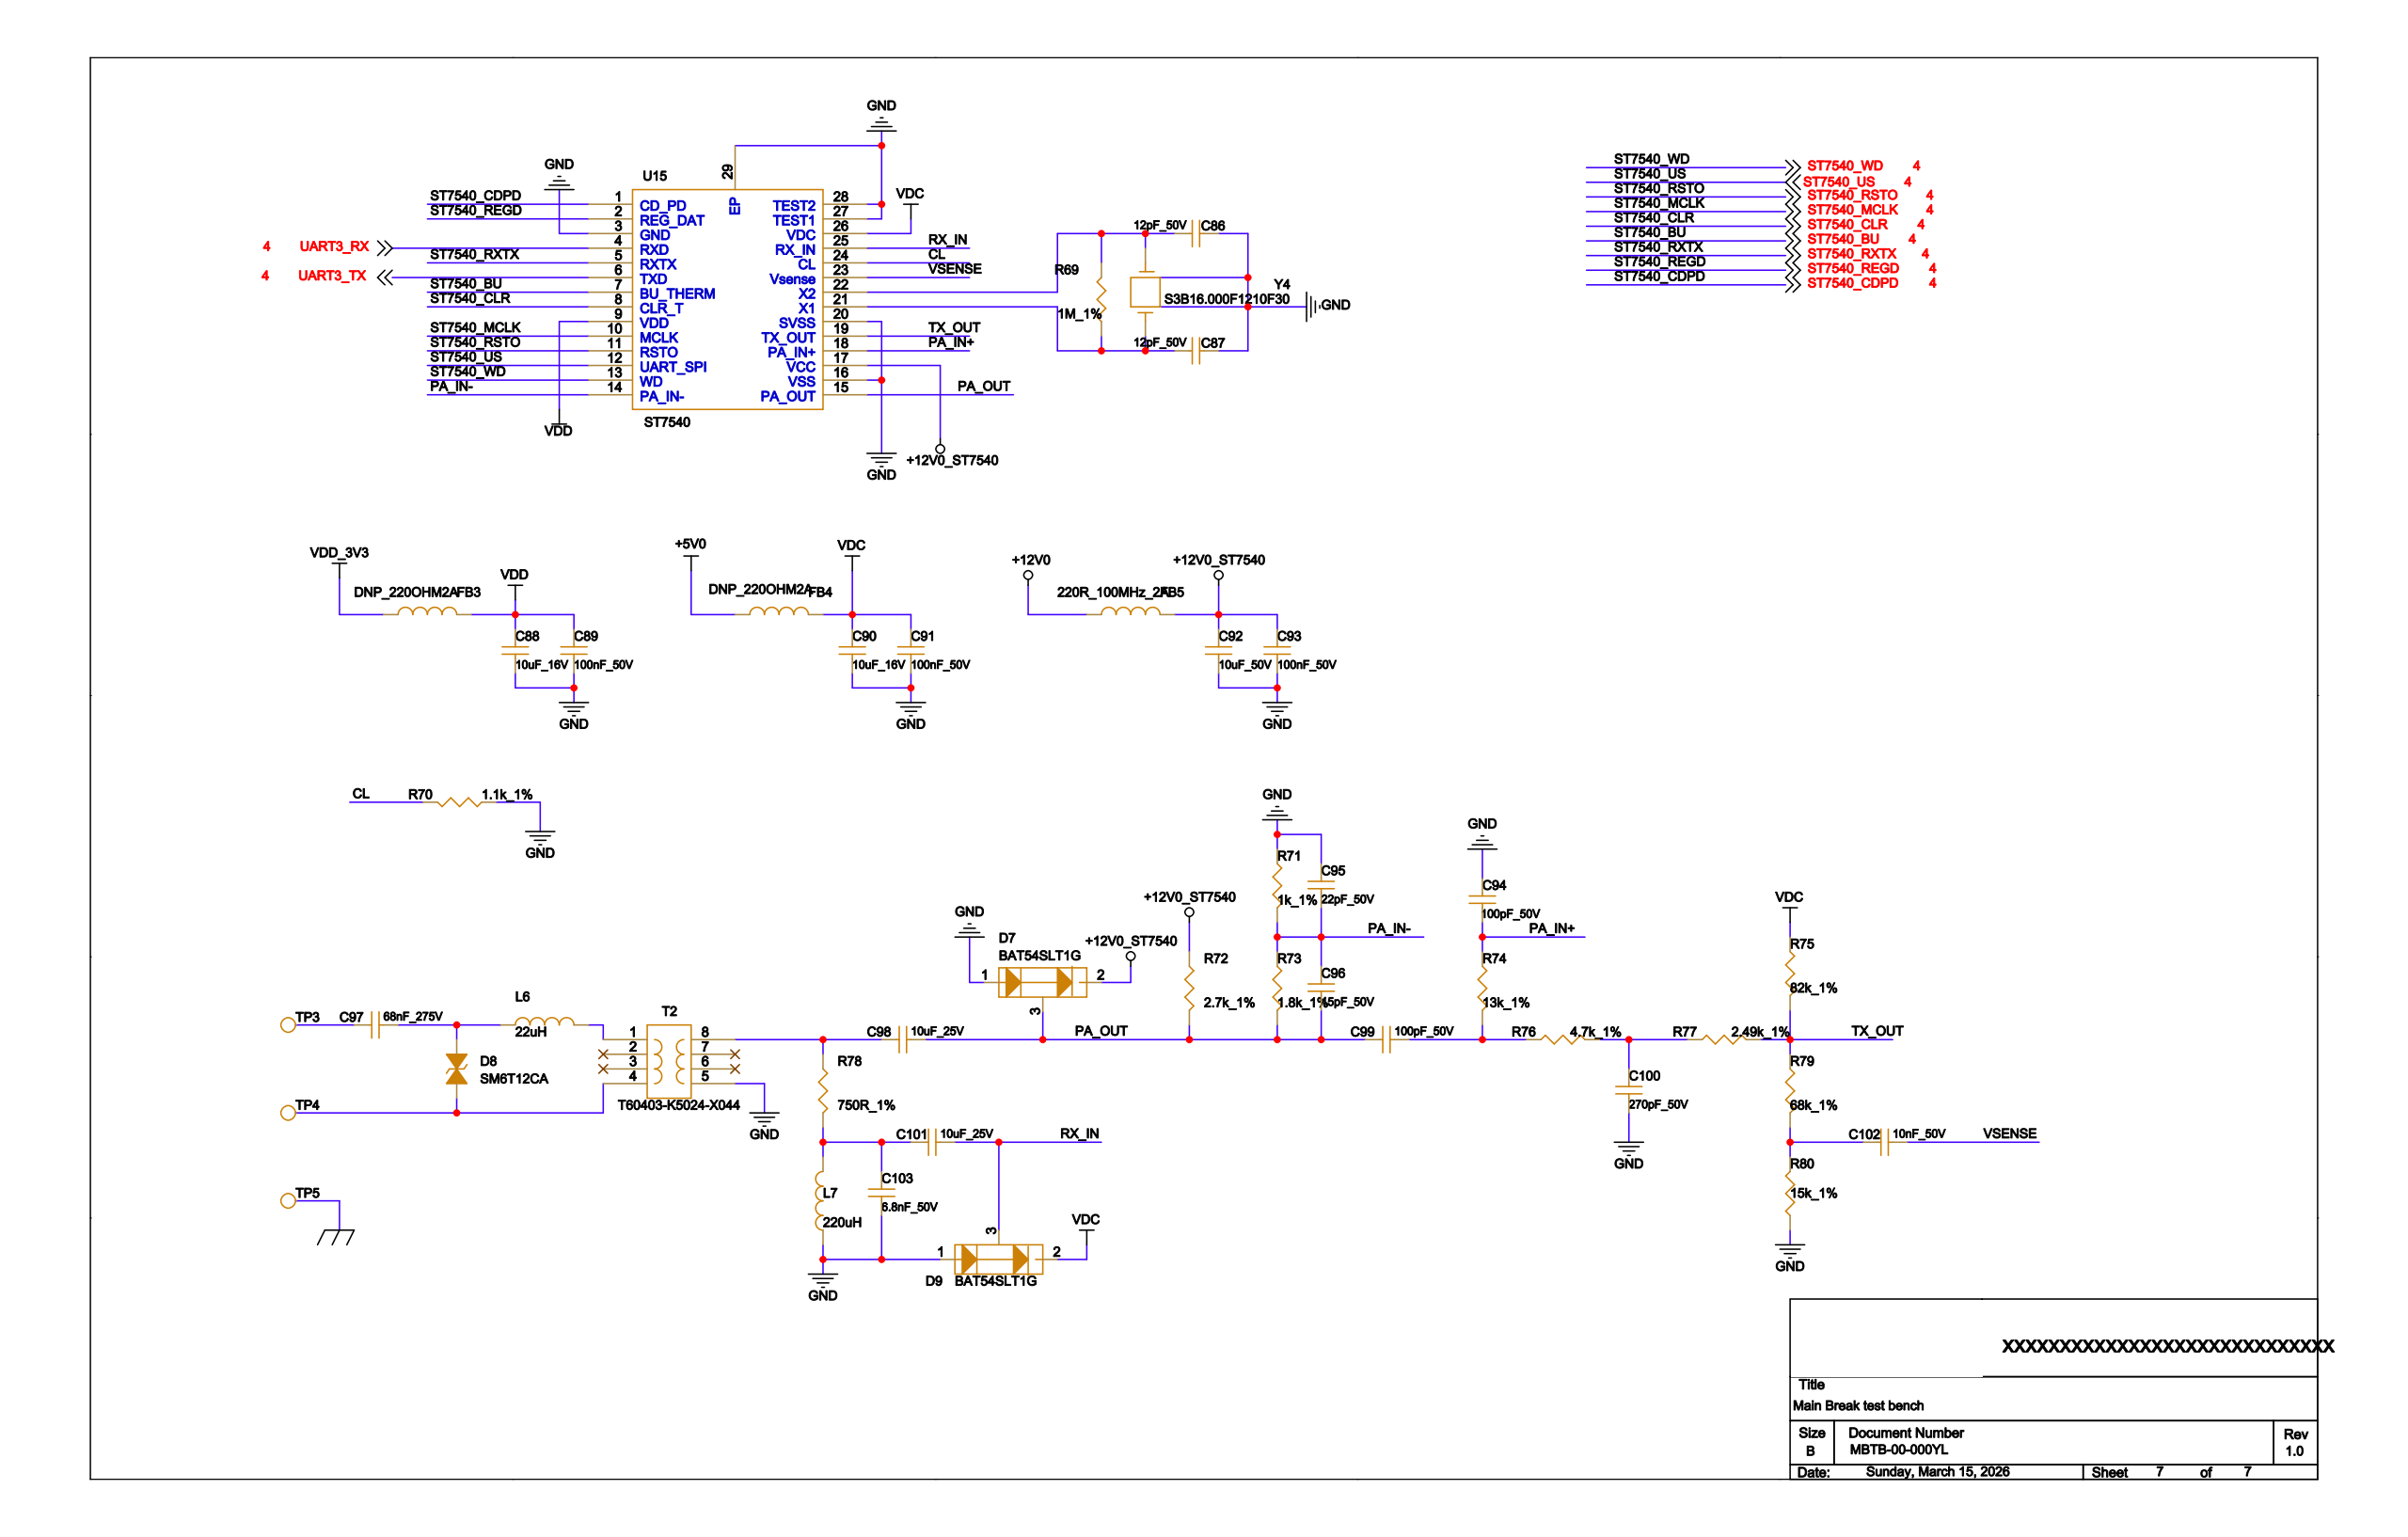Circuit board | Cadence Allegro | 260 parts | 211 nets | one sheet of the schematic
Parts on this sheet (reference | value | footprint):
C86 | 0603-C
C87 | 0603-C
C88 | 0603-C
C89 | 0603-C
C90 | 0603-C
C91 | 0603-C
C92 | 1206-C
C93 | 0603-C
C94 | 0603-C
C95 | 0603-C
C96 | 0603-C
C97 | CAP-TH_L13_0-W6_0-P10_00-D1_0
C98 | 1206-C
C99 | 0603-C
C100 | 0603-C
C101 | 1206-C
C102 | 0603-C
C103 | 1206-C
D7 | SOT23-3-0_95-H1_11
D8 | SMB
D9 | SOT23-3-0_95-H1_11
L6 | IND-SMD_L6_0-W6_0_B82462A4473K000
L7 | IND-SMD_L6_0-W6_0_B82462A4473K000
R69 | 0603-R
R70 | 0603-R
R71 | 0603-R
R72 | 0603-R
R73 | 0603-R
R74 | 0603-R
R75 | 0603-R
R76 | 0603-R
R77 | 0603-R
R78 | 1206-R
R79 | 0603-R
R80 | 0603-R
T2 | T60403-K5024-X044_VAC
TP3 | TP52_80
TP4 | TP52_80
TP5 | TP52_80
U15 | HTSSOP-28_L9_7-W4_4-P0_65-LS6_4-BL-EP
Y4 | X4-5_0X3_2-SG5032
Nets of these parts (net: part-pin ...):
N17252073: C86-1 R69-2 Y4-3 U15-22
GND: C86-2 C87-2 C88-2 C89-2 C90-2 C91-2 C92-2 C93-2 C94-1 C95-1 C100-2 C103-2 D7-1 D9-1 L7-1 R70-2 R71-2 R80-2 T2-5 Y4-2 Y4-4 U15-3 U15-16 U15-20 U15-27 U15-28 U15-29
N17252118: C87-1 R69-1 Y4-1 U15-21
CL: R70-1 U15-24
+12V0_ST7540: C92-1 C93-1 D7-2 R72-2 U15-17
N17261947: C100-1 R76-1 R77-2
N17255680: C101-1 C103-1 L7-2 R78-1
RX_IN: C101-2 D9-3 U15-25
N17258975: C98-1 R78-2 T2-8
PA_OUT: C96-2 C98-2 C99-1 D7-3 R72-1 R73-1 U15-15
N17262355: C102-1 R79-1 R80-1
VSENSE: C102-2 U15-23
GND_EARTH: TP5-1
VDD: C88-1 C89-1 U15-9
VDC: C90-1 C91-1 D9-2 R75-2 U15-26
PA_IN+: C94-2 R74-2 U15-18
N17261850: C99-2 R74-1 R76-2
PA_IN-: C95-2 C96-1 R71-1 R73-2 U15-14
N17255189: C97-1 TP3-1
N17255227: C97-2 D8-2 L6-1
N17255232: D8-1 T2-4 TP4-1
N17255367: L6-2 T2-1
TX_OUT: R75-1 R77-1 R79-2 U15-19
ST7540_BU: U15-7
ST7540_CDPD: U15-1
ST7540_CLR: U15-8
ST7540_MCLK: U15-10
ST7540_REGD: U15-2
ST7540_RSTO: U15-11
UART3_RX: U15-4
ST7540_RXTX: U15-5
UART3_TX: U15-6
ST7540_US: U15-12
ST7540_WD: U15-13